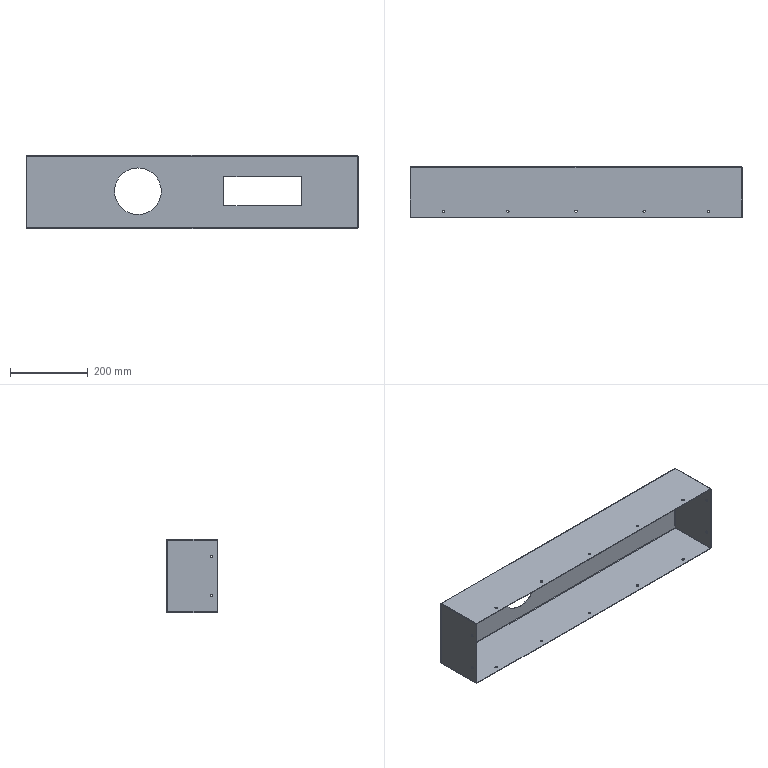Part | NX | features BREP 1 | 1 solid | 72 faces | box 854 x 130 x 189 mm | volume 598360 mm3 | cylinder 38 | plane 26 | spline 8 | commonest cylinder face diameters 6 x28 2 x4 5 x4 120 x2